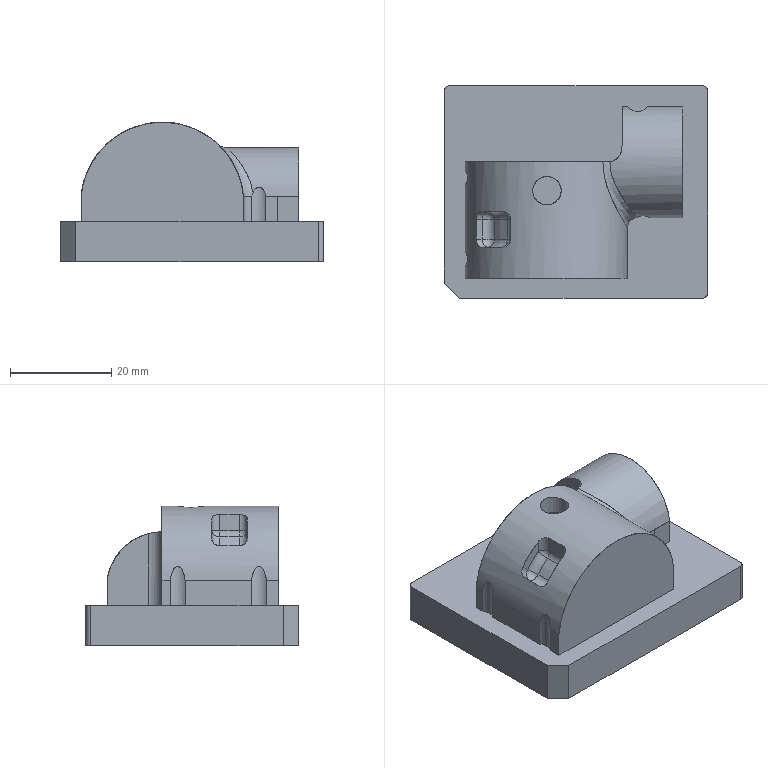NC program | PowerMill | posted with a generic post | part box 52 x 42 x 27.622 mm
Lines 8086 to 9073 of 214543:
N8183 M6
N8184 S18000 M03
N8185 G00 G90 X0.0 Y0.0
N8186 G43 Z9.8022 H2
N8187
N8188 G05 P10000 R4
N8189 X-11.2727 Y-8.4983
N8190 Z0.664
N8191 G01 Z-0.536 F3600.0
N8192 X-11.253 Y-8.5082 F6000.0
N8193 G03 X-10.9873 Y-8.4197 I0.0886 J0.1771
N8194 G01 X-10.3152 Y-7.0768
N8195 X-10.3131 Y-0.9761
N8196 X-10.3217 Y-0.4881
N8197 X-10.2511 Y0.0403
N8198 X-10.2223 Y0.1152
N8199 X-10.2021 Y0.1929
N8200 X-10.2026 Y0.2432
N8201 X-10.2153 Y0.2919
N8202 X-10.2491 Y0.39
N8203 X-10.3272 Y0.9761
N8204 X-10.2726 Y2.4403
N8205 X-10.3162 Y2.9283
N8206 X-10.3149 Y5.8566
N8207 X-10.271 Y6.3447
N8208 X-10.0887 Y6.8327
N8209 X-9.7611 Y7.2673
N8210 X-9.273 Y7.6166
N8211 X-8.7849 Y7.7804
N8212 X-8.5449 Y7.8088
N8213 X-3.2182
N8214 X-2.9283 Y7.7687
N8215 X-2.4403 Y7.5912
N8216 X-2.0533 Y7.3208
N8217 X-1.9522 Y7.217
N8218 X-1.672 Y6.8327
N8219 X-1.4899 Y6.3447
N8220 X-1.4465 Y5.8566
N8221 X-1.4524 Y3.4164
N8222 X-1.4311 Y2.9283
N8223 X-1.4486 Y2.4403
N8224 X-1.4344 Y1.4642
N8225 X-1.5424 Y0.9761
N8226 X-1.7966 Y0.4881
N8227 X-1.9197 Y0.3411
N8228 G03 X-1.915 Y0.0789 I0.1533 J-0.1284
N8229 G01 X-1.844 Y0.0
N8230 X-1.5621 Y-0.4881
N8231 X-1.4394 Y-0.9761
N8232 X-1.4309 Y-5.3686
N8233 X-1.4721 Y-11.7133
N8234 X-1.4462 Y-13.1774
N8235 X-1.4642 Y-13.5042
N8236 X-1.4978 Y-13.6655
N8237 X-1.5076 Y-16.5938
N8238 X-1.4799 Y-17.0818
N8239 X-1.5236 Y-17.5699
N8240 X-1.7078 Y-18.0579
N8241 X-1.9522 Y-18.3978
N8242 X-2.0901 Y-18.546
N8243 X-2.4403 Y-18.7916
N8244 X-2.9283 Y-18.982
N8245 X-3.4164 Y-19.0312
N8246 X-8.2969
N8247 X-8.7849 Y-18.9916
N8248 X-9.273 Y-18.8145
N8249 X-9.6626 Y-18.546
N8250 X-10.0487 Y-18.0579
N8251 X-10.2321 Y-17.5699
N8252 X-10.2757 Y-17.0818
N8253 X-10.2491 Y-16.7603
N8254 Y-13.7412
N8255 X-10.3174 Y-13.1774
N8256 X-10.3152 Y-7.0768
N8257 X-12.3194 Y-8.5465 Z-0.7339
N8258 X-12.2998 Y-8.5564
N8259 G03 X-12.0338 Y-8.4688 I0.0892 J0.1768
N8260 G01 X-11.3303 Y-7.0734
N8261 X-11.3083 Y-0.4881
N8262 X-11.341 Y0.4881
N8263 X-11.3376 Y1.9522
N8264 X-11.305 Y5.3686
N8265 X-11.3264 Y5.8566
N8266 X-11.2852 Y6.3447
N8267 X-11.1038 Y6.8327
N8268 X-10.7372 Y7.3041
N8269 X-10.2491 Y7.6361
N8270 X-9.7611 Y7.7863
N8271 X-9.5559 Y7.8088
N8272 X-2.2151
N8273 X-1.9522 Y7.776
N8274 X-1.4642 Y7.607
N8275 X-1.0506 Y7.3208
N8276 X-0.669 Y6.8327
N8277 X-0.4869 Y6.3447
N8278 X-0.4442 Y5.8566
N8279 X-0.4593 Y5.3686
N8280 X-0.4372 Y2.9283
N8281 X-0.4241 Y0.4881
N8282 X-0.4683 Y-0.4881
N8283 X-0.4694 Y-12.6894
N8284 X-0.4687 Y-12.6975
N8285 Y-12.6977
N8286 X-0.4287 Y-13.1774
N8287 X-0.4433 Y-17.0818
N8288 X-0.4874 Y-17.5699
N8289 X-0.6713 Y-18.0579
N8290 X-1.0566 Y-18.546
N8291 X-1.4642 Y-18.827
N8292 X-1.9522 Y-18.9954
N8293 X-2.4403 Y-19.0312
N8294 X-9.273
N8295 X-9.7611 Y-19.0038
N8296 X-10.2491 Y-18.8451
N8297 X-10.6981 Y-18.546
N8298 X-11.0831 Y-18.0579
N8299 X-11.2671 Y-17.5699
N8300 X-11.3123 Y-17.0818
N8301 Y-13.6655
N8302 X-11.3366 Y-13.1774
N8303 X-11.3039 Y-12.6894
N8304 Y-9.7611
N8305 X-11.3376 Y-9.273
N8306 X-11.3303 Y-7.0734
N8307 X-13.0764 Y-8.5492 Z-0.9319
N8308 X-13.0568 Y-8.5591
N8309 G03 X-12.7909 Y-8.4712 I0.089 J0.1769
N8310 G01 X-12.0869 Y-7.0716
N8311 X-12.0711 Y-0.4881
N8312 X-12.0926 Y0.4881
N8313 X-12.0688 Y1.9522
N8314 X-12.0711 Y5.3686
N8315 X-12.1008 Y5.8566
N8316 X-12.0572 Y6.3447
N8317 X-11.8757 Y6.8327
N8318 X-11.7133 Y7.0774
N8319 X-11.4951 Y7.3208
N8320 X-11.2252 Y7.5232
N8321 X-10.7372 Y7.7406
N8322 X-10.3258 Y7.8088
N8323 X-1.4166
N8324 X-0.9761 Y7.7318
N8325 X-0.4881 Y7.5019
N8326 X-0.2517 Y7.3208
N8327 X0.0 Y7.0353
N8328 X0.1291 Y6.8327
N8329 X0.3117 Y6.3447
N8330 X0.3535 Y5.8566
N8331 X0.3233 Y5.3686
N8332 X0.3174 Y2.4403
N8333 X0.3512 Y0.4881
N8334 X0.3285 Y-0.4881
N8335 Y-12.6894
N8336 X0.3501 Y-13.1774
N8337 X0.3226 Y-13.6655
N8338 Y-13.6714
N8339 X0.3364 Y-17.0818
N8340 X0.2924 Y-17.5699
N8341 X0.1097 Y-18.0579
N8342 X0.0 Y-18.2297
N8343 X-0.2743 Y-18.546
N8344 X-0.4881 Y-18.7104
N8345 X-0.9761 Y-18.9454
N8346 X-1.4642 Y-19.0295
N8347 X-2.4202 Y-19.0296
N8348 X-2.4403 Y-19.0311
N8349 X-9.273
N8350 X-9.2812 Y-19.0306
N8351 X-10.2491 Y-19.0308
N8352 X-10.7372 Y-18.9583
N8353 X-11.2252 Y-18.7393
N8354 X-11.4808 Y-18.546
N8355 X-11.7133 Y-18.2916
N8356 X-11.865 Y-18.0579
N8357 X-12.0489 Y-17.5699
N8358 X-12.0927 Y-17.0818
N8359 X-12.0773 Y-16.5938
N8360 X-12.0945 Y-13.1774
N8361 X-12.0711 Y-12.6894
N8362 Y-9.7611
N8363 X-12.0922 Y-9.273
N8364 X-12.0869 Y-7.0716
N8365 X-13.7539 Y-8.5524 Z-1.1299
N8366 X-13.7342 Y-8.5622
N8367 G03 X-13.4686 Y-8.4737 I0.0885 J0.1771
N8368 G01 X-12.7676 Y-7.0716
N8369 X-12.768 Y5.8566
N8370 X-12.7253 Y6.3447
N8371 X-12.543 Y6.8327
N8372 X-12.2013 Y7.2806
N8373 X-11.7133 Y7.6229
N8374 X-11.2252 Y7.7828
N8375 X-10.9964 Y7.8088
N8376 X-0.7671
N8377 X-0.4881 Y7.7728
N8378 X0.0 Y7.5993
N8379 X0.3964 Y7.3208
N8380 X0.7814 Y6.8327
N8381 X0.9612 Y6.3447
N8382 X1.0032 Y5.8566
N8383 X1.0097 Y0.4881
N8384 X0.9823 Y-0.4881
N8385 Y-12.6894
N8386 X0.9825 Y-12.6936
N8387 X1.0032 Y-13.1774
N8388 X0.9807 Y-13.6655
N8389 Y-16.5938
N8390 X1.0019 Y-17.0818
N8391 X0.9585 Y-17.5699
N8392 X0.7753 Y-18.0579
N8393 X0.3911 Y-18.546
N8394 X0.0 Y-18.8157
N8395 X-0.4881 Y-18.9922
N8396 X-0.9761 Y-19.0312
N8397 X-10.7372
N8398 X-11.2252 Y-19.0004
N8399 X-11.7133 Y-18.8375
N8400 X-12.1463 Y-18.546
N8401 X-12.5291 Y-18.0579
N8402 X-12.6894 Y-17.6582
N8403 X-12.7593 Y-17.0818
N8404 X-12.7343 Y-16.5938
N8405 Y-13.6655
N8406 X-12.7347 Y-13.6588
N8407 X-12.7674 Y-13.1774
N8408 X-12.7676 Y-7.0716
N8409 X-14.3135 Y-8.565 Z-1.3279
N8410 X-14.2939 Y-8.5749
N8411 G03 X-14.0278 Y-8.4877 I0.0895 J0.1766
N8412 G01 X-13.3091 Y-7.0688
N8413 X-13.3004 Y-5.3686
N8414 X-13.3058 Y5.3686
N8415 X-13.3302 Y5.8566
N8416 X-13.2882 Y6.3447
N8417 X-13.1774 Y6.6932
N8418 X-13.1083 Y6.8327
N8419 X-12.7282 Y7.3208
N8420 X-12.2013 Y7.6604
N8421 X-11.7133 Y7.7948
N8422 X-11.5628 Y7.8088
N8423 X-0.1929
N8424 X0.0 Y7.7882
N8425 X0.4881 Y7.6408
N8426 X0.9761 Y7.3146
N8427 X1.3529 Y6.8327
N8428 X1.4642 Y6.5808
N8429 X1.5353 Y6.3447
N8430 X1.5774 Y5.8566
N8431 X1.5492 Y5.3686
N8432 X1.5454 Y2.4403
N8433 X1.5729 Y0.4881
N8434 X1.5529 Y-0.4881
N8435 Y-0.4901
N8436 X1.5522 Y-6.8338
N8437 X1.5681 Y-13.1774
N8438 X1.5451 Y-13.6655
N8439 Y-13.6705
N8440 X1.5541 Y-17.0818
N8441 X1.5105 Y-17.5699
N8442 X1.3267 Y-18.0579
N8443 X0.9424 Y-18.546
N8444 X0.4881 Y-18.8479
N8445 X0.0 Y-19.0044
N8446 X-0.4881 Y-19.0312
N8447 X-11.2252
N8448 X-11.7133 Y-19.0105
N8449 X-12.2013 Y-18.8681
N8450 X-12.698 Y-18.546
N8451 X-13.0829 Y-18.0579
N8452 X-13.1774 Y-17.8526
N8453 X-13.2668 Y-17.5699
N8454 X-13.3097 Y-17.0818
N8455 X-13.2998 Y-16.5938
N8456 X-13.3155 Y-13.1774
N8457 X-13.2967 Y-12.6894
N8458 Y-9.7611
N8459 X-13.3205 Y-9.273
N8460 X-13.3091 Y-7.0688
N8461 X-14.8404 Y-8.5748 Z-1.5258
N8462 X-14.8208 Y-8.5847
N8463 G03 X-14.5551 Y-8.4963 I0.0887 J0.1771
N8464 G01 X-13.8402 Y-7.0685
N8465 X-13.8331 Y5.8566
N8466 X-13.7893 Y6.3447
N8467 X-13.6075 Y6.8327
N8468 X-13.2258 Y7.3208
N8469 X-12.6894 Y7.6636
N8470 X-12.2013 Y7.7962
N8471 X-11.6919 Y7.7967
N8472 X-11.5628 Y7.8088
N8473 X-0.1929
N8474 X-0.1863 Y7.8085
N8475 X-0.1796 Y7.8084
N8476 X0.3068 Y7.8088
N8477 X0.4881 Y7.7899
N8478 X0.9761 Y7.6461
N8479 X1.4711 Y7.3208
N8480 X1.8528 Y6.8327
N8481 X1.9522 Y6.61
N8482 X2.0345 Y6.3447
N8483 X2.0765 Y5.8566
N8484 X2.085 Y0.4881
N8485 X2.0547 Y-0.4881
N8486 Y-12.6894
N8487 X2.085 Y-13.1774
N8488 X2.0855 Y-17.0818
N8489 X2.0407 Y-17.5699
N8490 X1.9522 Y-17.8552
N8491 X1.8579 Y-18.0579
N8492 X1.4736 Y-18.546
N8493 X0.9761 Y-18.869
N8494 X0.4881 Y-19.0104
N8495 X0.0 Y-19.0312
N8496 X-11.7133
N8497 X-12.2013 Y-19.0166
N8498 X-12.6894 Y-18.8886
N8499 X-13.1774 Y-18.5908
N8500 X-13.6127 Y-18.0579
N8501 X-13.7977 Y-17.5699
N8502 X-13.842 Y-17.0818
N8503 X-13.8432 Y-13.1774
N8504 X-13.8222 Y-12.6894
N8505 Y-9.7611
N8506 X-13.8414 Y-9.273
N8507 X-13.8402 Y-7.0685
N8508 X-15.2983 Y-8.5761 Z-1.7238
N8509 X-15.2787 Y-8.586
N8510 G03 X-15.013 Y-8.4975 I0.0886 J0.1771
N8511 G01 X-14.2981 Y-7.0684
N8512 X-14.2968 Y-1.4642
N8513 X-14.2849 Y0.9761
N8514 X-14.3027 Y5.8566
N8515 X-14.2625 Y6.3447
N8516 X-14.0801 Y6.8327
N8517 X-13.6982 Y7.3208
N8518 X-13.1774 Y7.658
N8519 X-12.6894 Y7.7939
N8520 X-12.5336 Y7.8088
N8521 X0.7777
N8522 X0.9761 Y7.7873
N8523 X1.4642 Y7.6377
N8524 X1.9426 Y7.3208
N8525 X2.3239 Y6.8327
N8526 X2.4403 Y6.5697
N8527 X2.506 Y6.3447
N8528 X2.5483 Y5.8566
N8529 X2.538 Y2.9275
N8530 Y2.9267
N8531 X2.5511 Y0.0
N8532 X2.5517 Y-13.1774
N8533 X2.5198 Y-13.6655
N8534 X2.5305 Y-17.0818
N8535 X2.487 Y-17.5699
N8536 X2.3032 Y-18.0579
N8537 X1.9189 Y-18.546
N8538 X1.4642 Y-18.8489
N8539 X0.9761 Y-19.0045
N8540 X0.4881 Y-19.0312
N8541 X-12.2013
N8542 X-12.6894 Y-19.0106
N8543 X-13.1774 Y-18.8693
N8544 X-13.6744 Y-18.546
N8545 X-14.0587 Y-18.0579
N8546 X-14.1535 Y-17.8499
N8547 X-14.2424 Y-17.5699
N8548 X-14.2861 Y-17.0818
N8549 X-14.2737 Y-13.6655
N8550 X-14.2941 Y-13.1774
N8551 X-14.2985 Y-9.273
N8552 X-14.2981 Y-7.0684
N8553 X-15.7274 Y-8.5633 Z-1.9218
N8554 X-15.7078 Y-8.5732
N8555 G03 X-15.4418 Y-8.4857 I0.0892 J0.1767
N8556 G01 X-14.7257 Y-7.0668
N8557 X-14.7083 Y-2.4403
N8558 X-14.7155 Y5.8566
N8559 X-14.6729 Y6.3447
N8560 X-14.4913 Y6.8327
N8561 X-14.1535 Y7.2779
N8562 X-13.6655 Y7.622
N8563 X-13.1774 Y7.782
N8564 X-12.6894 Y7.8113
N8565 X1.2014 Y7.8088
N8566 X1.4642 Y7.7759
N8567 X1.9522 Y7.6057
N8568 X2.4403 Y7.2488
N8569 X2.7466 Y6.8327
N8570 X2.9288 Y6.3447
N8571 X2.9705 Y5.8566
N8572 X2.9532 Y5.3686
N8573 Y5.365
N8574 X2.9593 Y0.9761
N8575 X2.953 Y-0.4881
N8576 Y-12.6894
N8577 X2.9532 Y-12.6932
N8578 X2.9715 Y-13.1774
N8579 X2.9684 Y-17.0818
N8580 X2.9249 Y-17.5699
N8581 X2.741 Y-18.0579
N8582 X2.3567 Y-18.546
N8583 X1.9522 Y-18.8241
N8584 X1.4642 Y-18.995
N8585 X0.9761 Y-19.0312
N8586 X-12.6894
N8587 X-13.1774 Y-19.003
N8588 X-13.6655 Y-18.8465
N8589 X-14.1123 Y-18.546
N8590 X-14.4966 Y-18.0579
N8591 X-14.6802 Y-17.5699
N8592 X-14.7239 Y-17.0818
N8593 X-14.7073 Y-10.2491
N8594 X-14.734 Y-9.273
N8595 X-14.7257 Y-7.0668
N8596 X-15.8149 Y-8.6426 Z-2.1198
N8597 X-15.7952 Y-8.6524
N8598 G03 X-15.5295 Y-8.564 I0.0886 J0.177
N8599 G01 X-14.78 Y-7.0668
N8600 X-14.7793 Y-5.66
N8601 X-14.7869 Y-5.6054
N8602 X-14.809 Y-5.5549
N8603 X-14.9239 Y-5.3686
N8604 X-15.0957 Y-4.8805
N8605 X-15.1296 Y-4.6055
N8606 X-15.1254 Y-3.9044
N8607 Y-3.9038
N8608 X-15.1253 Y5.8566
N8609 X-15.0855 Y6.3447
N8610 X-14.9031 Y6.8327
N8611 X-14.6416 Y7.1993
N8612 X-14.5225 Y7.3208
N8613 X-14.1535 Y7.583
N8614 X-13.6655 Y7.7668
N8615 X-13.1774 Y7.8113
N8616 X-12.6899 Y7.8112
N8617 X-12.6894 Y7.8113
N8618 X-9.7699 Y7.8107
N8619 X1.6056 Y7.8088
N8620 X1.9522 Y7.7574
N8621 X2.4403 Y7.5615
N8622 X2.7696 Y7.3208
N8623 X2.9283 Y7.1559
N8624 X3.1516 Y6.8327
N8625 X3.3342 Y6.3447
N8626 X3.3743 Y5.8566
N8627 X3.377 Y2.9283
N8628 X3.3555 Y-0.4881
N8629 Y-12.6894
N8630 X3.3741 Y-13.1774
N8631 X3.3657 Y-17.0818
N8632 X3.3206 Y-17.5699
N8633 X3.1362 Y-18.0579
N8634 X2.9283 Y-18.3607
N8635 X2.7522 Y-18.546
N8636 X2.4403 Y-18.7733
N8637 X1.9522 Y-18.9728
N8638 X1.4642 Y-19.0312
N8639 X-13.1774
N8640 X-13.6655 Y-18.9841
N8641 X-14.1535 Y-18.7977
N8642 X-14.5075 Y-18.546
N8643 X-14.6416 Y-18.4102
N8644 X-14.8918 Y-18.0579
N8645 X-15.0756 Y-17.5699
N8646 X-15.1206 Y-17.0818
N8647 X-15.1314 Y-10.2491
N8648 X-15.0501 Y-9.7611
N8649 X-14.8016 Y-9.2556
N8650 X-14.7862 Y-9.2127
N8651 X-14.781 Y-9.1675
N8652 X-14.78 Y-7.0668
N8653 X-16.0588 Y-9.1299 Z-2.3177
N8654 X-16.0391 Y-9.1398
N8655 G03 X-15.7735 Y-9.0513 I0.0886 J0.1771
N8656 G01 X-14.7799 Y-7.0668
N8657 X-14.7793 Y-5.7347
N8658 X-14.7957 Y-5.6571
N8659 X-14.8409 Y-5.592
N8660 X-15.074 Y-5.3686
N8661 X-15.3674 Y-4.8805
N8662 X-15.4919 Y-4.3925
N8663 X-15.4877 Y0.7321
N8664 X-15.4943 Y5.8566
N8665 X-15.4522 Y6.3447
N8666 X-15.2701 Y6.8327
N8667 X-15.1296 Y7.0508
N8668 X-14.8888 Y7.3208
N8669 X-14.6416 Y7.511
N8670 X-14.1535 Y7.7341
N8671 X-13.724 Y7.8088
N8672 X-13.2038
N8673 X-13.1774 Y7.8113
N8674 X-12.6899 Y7.8112
N8675 X-12.6894
N8676 X-9.7699 Y7.8107
N8677 X1.305 Y7.8088
N8678 X1.974
N8679 X2.4403 Y7.7235
N8680 X2.9283 Y7.4859
N8681 X3.139 Y7.3208
N8682 X3.4164 Y6.9992
N8683 X3.5203 Y6.8327
N8684 X3.7021 Y6.3447
N8685 X3.7453 Y5.8566
N8686 X3.7327 Y5.3686
N8687 X3.7465 Y0.0
N8688 X3.7477 Y-13.1774
N8689 X3.7222 Y-13.6655
N8690 X3.7297 Y-17.0818
N8691 X3.687 Y-17.5699
N8692 X3.5033 Y-18.0579
N8693 X3.4164 Y-18.1987
N8694 X3.1189 Y-18.546
N8695 X2.9283 Y-18.697
N8696 X2.4403 Y-18.9391
N8697 X1.9522 Y-19.0288
N8698 X1.4832
N8699 X1.4642 Y-19.0311
N8700 X-13.1774
N8701 X-13.1883 Y-19.0301
N8702 X-13.6655
N8703 X-14.1535 Y-18.9518
N8704 X-14.6416 Y-18.7244
N8705 X-14.8747 Y-18.546
N8706 X-15.1296 Y-18.2582
N8707 X-15.259 Y-18.0579
N8708 X-15.4426 Y-17.5699
N8709 X-15.4862 Y-17.0818
N8710 X-15.4777 Y-16.5938
N8711 X-15.5061 Y-10.7372
N8712 X-15.4597 Y-10.2491
N8713 X-15.2769 Y-9.7611
N8714 X-15.1296 Y-9.5298
N8715 X-14.837 Y-9.2325
N8716 X-14.8099 Y-9.198
N8717 X-14.8003 Y-9.1782
N8718 X-14.7859 Y-9.1367
N8719 X-14.7809 Y-9.0931
N8720 X-14.7799 Y-7.0668
N8721 X-16.8357 Y-10.6818 Z-2.5157
N8722 X-16.816 Y-10.6917
N8723 G03 X-16.5503 Y-10.6032 I0.0886 J0.1771
N8724 G01 X-14.7799 Y-7.0668
N8725 X-14.7793 Y-5.8144
N8726 X-14.7812 Y-5.8007
N8727 X-14.8135 Y-5.703
N8728 X-14.8912 Y-5.6355
N8729 X-15.2602 Y-5.3686
N8730 X-15.6177 Y-4.9112
N8731 X-15.8131 Y-4.3925
N8732 X-15.8552 Y-3.9044
N8733 X-15.8311 Y-1.9522
N8734 X-15.836 Y5.8566
N8735 X-15.7939 Y6.3447
N8736 X-15.6118 Y6.8327
N8737 X-15.2305 Y7.3208
N8738 X-15.1296 Y7.4058
N8739 X-14.6416 Y7.6849
N8740 X-14.1535 Y7.8007
N8741 X-13.7695 Y7.8009
N8742 X-13.724 Y7.8088
N8743 X-13.2038
N8744 X-13.1774 Y7.8112
N8745 X-12.6899 Y7.8111
N8746 X-12.6894 Y7.8112
N8747 X-9.7699 Y7.8106
N8748 X1.305 Y7.8088
N8749 X1.974
N8750 X1.9747 Y7.8087
N8751 X2.3243 Y7.8088
N8752 X2.9283 Y7.6743
N8753 X3.4898 Y7.3208
N8754 X3.8697 Y6.8327
N8755 X4.0525 Y6.3447
N8756 X4.0943 Y5.8566
N8757 X4.0768 Y5.3686
N8758 X4.0818 Y0.9761
N8759 X4.0774 Y-0.4881
N8760 Y-12.6894
N8761 X4.0964 Y-17.0818
N8762 X4.055 Y-17.5699
N8763 X3.9044 Y-17.9918
N8764 X3.4869 Y-18.546
N8765 X2.9283 Y-18.8956
N8766 X2.4403 Y-19.0187
N8767 X1.9522 Y-19.0312
N8768 X-13.6655
N8769 X-14.1535 Y-19.0232
N8770 X-14.6416 Y-18.9119
N8771 X-15.1296 Y-18.64
N8772 X-15.2424 Y-18.546
N8773 X-15.6177 Y-18.0734
N8774 X-15.8104 Y-17.5699
N8775 X-15.8538 Y-17.0818
N8776 X-15.8346 Y-16.5938
N8777 X-15.8303 Y-12.6894
N8778 X-15.8529 Y-10.7372
N8779 X-15.7624 Y-10.2491
N8780 X-15.6177 Y-9.9165
N8781 X-15.5226 Y-9.7611
N8782 X-15.1296 Y-9.3475
N8783 X-14.8743 Y-9.1899
N8784 X-14.811 Y-9.1278
N8785 X-14.7809 Y-9.0444
N8786 X-14.7799 Y-7.0668
N8787 X-16.1848 Y-8.57 Z-2.7137
N8788 X-16.1652 Y-8.5799
N8789 G03 X-15.8995 Y-8.4915 I0.0887 J0.1771
N8790 G01 X-14.7794 Y-6.2542
N8791 X-14.7793 Y-5.9105
N8792 X-14.793 Y-5.8038
N8793 X-14.857 Y-5.7174
N8794 X-14.9101 Y-5.688
N8795 X-14.9242 Y-5.6828
N8796 X-15.1296 Y-5.607
N8797 X-15.5051 Y-5.3686
N8798 X-15.6177 Y-5.2674
N8799 X-15.9258 Y-4.8805
N8800 X-16.1057 Y-4.4641
N8801 X-16.1866 Y-3.9044
N8802 X-16.1777 Y5.8566
N8803 X-16.1356 Y6.3447
N8804 X-15.9535 Y6.8327
N8805 X-15.6177 Y7.2759
N8806 X-15.1296 Y7.6217
N8807 X-14.6416 Y7.7816
N8808 X-14.1535 Y7.8113
N8809 X-12.6896 Y7.8111
N8810 X-12.6894
N8811 X-12.2274 Y7.811
N8812 X2.6576 Y7.8088
N8813 X2.9283 Y7.7745
N8814 X3.4164 Y7.6034
N8815 X3.8234 Y7.3208
N8816 X4.2039 Y6.8327
N8817 X4.3862 Y6.3447
N8818 X4.4288 Y5.8566
N8819 X4.4317 Y0.4881
N8820 X4.4083 Y-0.4881
N8821 Y-12.6894
N8822 X4.43 Y-13.1774
N8823 X4.4299 Y-17.0818
N8824 X4.3925 Y-17.5296
N8825 X4.2008 Y-18.0579
N8826 X3.8165 Y-18.546
N8827 X3.4164 Y-18.8229
N8828 X2.9283 Y-18.9943
N8829 X2.4403 Y-19.0312
N8830 X-14.1535
N8831 X-14.6416 Y-19.0018
N8832 X-15.1296 Y-18.8437
N8833 X-15.5721 Y-18.546
N8834 X-15.955 Y-18.0579
N8835 X-16.1394 Y-17.5699
N8836 X-16.1852 Y-17.0818
N8837 X-16.1876 Y-13.9095
N8838 X-16.1785 Y-10.7372
N8839 X-16.068 Y-10.2491
N8840 X-15.7988 Y-9.7611
N8841 X-15.6177 Y-9.5586
N8842 X-15.2386 Y-9.273
N8843 X-14.9043 Y-9.1379
N8844 X-14.8206 Y-9.0742
N8845 X-14.7808 Y-8.9768
N8846 X-14.7794 Y-6.2542
N8847 X-16.5683 Y-6.1914 Z-2.9117
N8848 X-16.5464 Y-6.1928
N8849 G03 X-16.3368 Y-6.0071 I0.012 J0.1977
N8850 G01 X-16.2629 Y-4.79
N8851 X-16.4324 Y-4.3925
N8852 X-16.4953 Y-3.9044
N8853 X-16.4968 Y5.8566
N8854 X-16.4532 Y6.3447
N8855 X-16.2708 Y6.8327
N8856 X-16.1057 Y7.085
N8857 X-15.8894 Y7.3208
N8858 X-15.6177 Y7.5262
N8859 X-15.1296 Y7.7419
N8860 X-14.7236 Y7.8088
N8861 X-14.1931
N8862 X-14.1535 Y7.8113
N8863 X-12.6896 Y7.811
N8864 X-12.6894 Y7.8111
N8865 X-12.2274 Y7.811
N8866 X2.3159 Y7.8088
N8867 X2.9695
N8868 X3.4164 Y7.7302
N8869 X3.9044 Y7.5003
N8870 X4.1343 Y7.3208
N8871 X4.3925 Y7.0271
N8872 X4.5157 Y6.8327
N8873 X4.6978 Y6.3447
N8874 X4.7405 Y5.8566
N8875 X4.7393 Y-12.2013
N8876 X4.7248 Y-13.6655
N8877 X4.7283 Y-17.0818
N8878 X4.6846 Y-17.5699
N8879 X4.501 Y-18.0579
N8880 X4.3925 Y-18.2323
N8881 X4.1164 Y-18.546
N8882 X3.9044 Y-18.7114
N8883 X3.4164 Y-18.9452
N8884 X2.9283 Y-19.0296
N8885 X2.4595 Y-19.0297
N8886 X2.4403 Y-19.0311
N8887 X-14.1535
N8888 X-14.1573 Y-19.031
N8889 X-14.161
N8890 X-14.6416
N8891 X-15.1296 Y-18.9573
N8892 X-15.6177 Y-18.7385
N8893 X-15.8722 Y-18.546
N8894 X-16.1057 Y-18.2896
N8895 X-16.257 Y-18.0579
N8896 X-16.4401 Y-17.5699
N8897 X-16.4839 Y-17.0818
N8898 X-16.4861 Y-10.7372
N8899 X-16.3691 Y-10.2491
N8900 X-16.0907 Y-9.7611
N8901 X-15.6177 Y-9.3407
N8902 X-15.503 Y-9.273
N8903 X-15.1296 Y-9.1241
N8904 X-14.9441 Y-9.0905
N8905 G03 X-14.7807 Y-8.9123 I-0.0357 J0.1968
N8906 G01 X-14.7793 Y-6.1448
N8907 Y-5.9414
N8908 G03 X-14.9432 Y-5.7446 I-0.2 J0.0001
N8909 G01 X-15.1296 Y-5.7105
N8910 X-15.6177 Y-5.4954
N8911 X-15.7964 Y-5.3686
N8912 X-16.1057 Y-5.0505
N8913 X-16.2243 Y-4.8805
N8914 X-16.2629 Y-4.79
N8915 X-16.8452 Y-6.2207 Z-3.1096
N8916 X-16.8232 Y-6.222
N8917 G03 X-16.6136 Y-6.0364 I0.012 J0.1976
N8918 G01 X-16.54 Y-4.8258
N8919 X-16.7247 Y-4.3925
N8920 X-16.7877 Y-3.9044
N8921 X-16.7815 Y5.8566
N8922 X-16.7395 Y6.3447
N8923 X-16.5938 Y6.759
N8924 X-16.1763 Y7.3208
N8925 X-15.6177 Y7.6722
N8926 X-15.1296 Y7.7988
N8927 X-15.0112 Y7.8088
N8928 X-14.7315 Y7.8086
N8929 X-14.7275 Y7.8087
N8930 X-14.7236 Y7.8088
N8931 X-14.1931
N8932 X-14.1535 Y7.8112
N8933 X-12.6896 Y7.811
N8934 X-12.6894
N8935 X-12.2274 Y7.8109
N8936 X2.3159 Y7.8088
N8937 X2.9695
N8938 X3.0442 Y7.7957
N8939 X3.4164 Y7.7954
N8940 X3.9044 Y7.6613
N8941 X4.3925 Y7.3589
N8942 X4.817 Y6.8327
N8943 X4.9991 Y6.3447
N8944 X5.0413 Y5.8566
N8945 X5.0236 Y5.3686
N8946 X5.0305 Y0.0
N8947 Y-12.6894
N8948 X5.0197 Y-16.5938
N8949 X5.0419 Y-17.0818
N8950 X4.9976 Y-17.5699
N8951 X4.8145 Y-18.0579
N8952 X4.4287 Y-18.546
N8953 X3.9044 Y-18.8821
N8954 X3.4164 Y-19.0142
N8955 X2.9283 Y-19.0312
N8956 X-14.6416
N8957 X-15.1296 Y-19.0201
N8958 X-15.6177 Y-18.8996
N8959 X-16.1057 Y-18.6135
N8960 X-16.1858 Y-18.546
N8961 X-16.5701 Y-18.0579
N8962 X-16.7529 Y-17.5699
N8963 X-16.7974 Y-17.0818
N8964 X-16.7753 Y-16.5938
N8965 X-16.7784 Y-10.7372
N8966 X-16.6615 Y-10.2491
N8967 X-16.5938 Y-10.096
N8968 X-16.3826 Y-9.7611
N8969 X-16.1057 Y-9.4812
N8970 X-15.7954 Y-9.273
N8971 X-15.6177 Y-9.1915
N8972 X-15.1296 Y-9.0675
N8973 X-14.9718 Y-9.0616
N8974 G03 X-14.7806 Y-8.8841 I-0.0076 J0.1999
N8975 G01 X-14.7793 Y-6.1161
N8976 Y-5.9739
N8977 G03 X-14.9722 Y-5.7741 I-0.2 J0.0
N8978 G01 X-15.1296 Y-5.7684
N8979 X-15.6177 Y-5.6438
N8980 X-16.0889 Y-5.3686
N8981 X-16.5167 Y-4.8805
N8982 X-16.54 Y-4.8258
N8983 X-17.1306 Y-6.2387 Z-3.3076
N8984 X-17.1086 Y-6.24
N8985 G03 X-16.899 Y-6.0544 I0.012 J0.1976
N8986 G01 X-16.8252 Y-4.8426
N8987 X-17.0171 Y-4.3925
N8988 X-17.0801 Y-3.9044
N8989 X-17.074 Y5.8566
N8990 X-17.032 Y6.3447
N8991 X-16.8499 Y6.8327
N8992 X-16.5938 Y7.1933
N8993 X-16.4684 Y7.3208
N8994 X-16.1057 Y7.5792
N8995 X-15.6177 Y7.7644
N8996 X-15.1296 Y7.8113
N8997 X3.5535 Y7.8088
N8998 X3.9044 Y7.7565
N8999 X4.3925 Y7.5593
N9000 X4.7186 Y7.3208
N9001 X4.8805 Y7.1512
N9002 X5.1014 Y6.8327
N9003 X5.2818 Y6.3447
N9004 X5.324 Y5.8566
N9005 X5.3075 Y-0.4881
N9006 Y-12.6894
N9007 X5.3157 Y-17.0818
N9008 X5.2718 Y-17.5699
N9009 X5.088 Y-18.0579
N9010 X4.8805 Y-18.3592
N9011 X4.7046 Y-18.546
N9012 X4.3925 Y-18.7739
N9013 X3.9044 Y-18.9732
N9014 X3.4164 Y-19.0312
N9015 X-15.1296
N9016 X-15.6177 Y-18.9842
N9017 X-16.1057 Y-18.7976
N9018 X-16.4592 Y-18.546
N9019 X-16.5938 Y-18.408
N9020 X-16.8435 Y-18.0579
N9021 X-17.0282 Y-17.5699
N9022 X-17.0716 Y-17.0818
N9023 X-17.0708 Y-10.7372
N9024 X-16.954 Y-10.2491
N9025 X-16.6745 Y-9.7611
N9026 X-16.5938 Y-9.6671
N9027 X-16.1057 Y-9.2836
N9028 X-15.6177 Y-9.0994
N9029 X-15.1296 Y-9.0544
N9030 X-14.9801 Y-9.0543
N9031 G03 X-14.7806 Y-8.8462 I0.0002 J0.1995
N9032 G01 X-14.7796 Y-6.7704
N9033 X-14.7793 Y-5.9809
N9034 G03 X-14.9791 Y-5.7809 I-0.2 J0.0
N9035 G01 X-15.1296 Y-5.7807
N9036 X-15.6177 Y-5.7351
N9037 X-16.1057 Y-5.5517
N9038 X-16.3814 Y-5.3686
N9039 X-16.5938 Y-5.1679
N9040 X-16.8091 Y-4.8805
N9041 X-16.8252 Y-4.8426
N9042 X-17.3981 Y-6.2498 Z-3.5056
N9043 X-17.3761 Y-6.2511
N9044 G03 X-17.167 Y-6.0648 I0.0114 J0.1977
N9045 G01 X-17.097 Y-4.854
N9046 X-17.2953 Y-4.3925
N9047 X-17.3585 Y-3.9044
N9048 X-17.3483 Y0.9761
N9049 X-17.3501 Y5.8566
N9050 X-17.3076 Y6.3447
N9051 X-17.1262 Y6.8327
N9052 X-16.7449 Y7.3208
N9053 X-16.5938 Y7.4441
N9054 X-16.1057 Y7.7036
N9055 X-15.6177 Y7.8057
N9056 X-15.1867 Y7.8058
N9057 X-15.1296 Y7.8113
N9058 X3.5331 Y7.8088
N9059 X3.8279
N9060 X4.3925 Y7.6904
N9061 X4.8805 Y7.4162
N9062 X4.9944 Y7.3208
N9063 X5.3686 Y6.8425
N9064 X5.558 Y6.3447
N9065 X5.6017 Y5.8566
N9066 X5.5846 Y0.0
N9067 Y-12.6894
N9068 X5.5974 Y-17.0818
N9069 X5.5522 Y-17.5699
N9070 X5.3686 Y-18.0575
N9071 X4.9843 Y-18.546
N9072 X4.8805 Y-18.6321
N9073 X4.3925 Y-18.9076
N9074 X3.9044 Y-19.0226
N9075 X3.4164 Y-19.0312
N9076 X-15.1296
N9077 X-15.6177 Y-19.0259
N9078 X-16.1057 Y-18.9238
N9079 X-16.5938 Y-18.6649
N9080 X-16.7396 Y-18.546
N9081 X-17.0818 Y-18.1292
N9082 X-17.3075 Y-17.5699
N9083 X-17.3527 Y-17.0818
N9084 X-17.3483 Y-10.7372
N9085 X-17.2315 Y-10.2491
N9086 X-17.0818 Y-9.9477
N9087 X-16.9523 Y-9.7611
N9088 X-16.5938 Y-9.4173
N9089 X-16.3658 Y-9.273
N9090 X-16.1057 Y-9.1591
N9091 X-15.6177 Y-9.0588
N9092 X-15.2691 Y-9.0589
N9093 X-14.9208 Y-9.0454
N9094 G03 X-14.7805 Y-8.8675 I-0.0593 J0.1911
N9095 G01 X-14.7796 Y-7.011
N9096 X-14.7793 Y-5.9919
N9097 X-14.7803 Y-5.972
N9098 X-14.7833 Y-5.9524
N9099 G03 X-14.9791 Y-5.7808 I-0.194 J-0.0238
N9100 G01 X-15.1296 Y-5.7807
N9101 X-15.1504 Y-5.7787
N9102 X-15.6177 Y-5.7758
N9103 X-16.1057 Y-5.6759
N9104 X-16.5938 Y-5.4183
N9105 X-17.0818 Y-4.8892
N9106 X-17.097 Y-4.854
N9107 X-17.6681 Y-6.2269 Z-3.7036
N9108 X-17.6461 Y-6.2283
N9109 G03 X-17.4363 Y-6.0428 I0.0121 J0.1976
N9110 G01 X-17.362 Y-4.8317
N9111 X-17.5489 Y-4.3925
N9112 X-17.6123 Y-3.9044
N9113 X-17.6127 Y5.8566
N9114 X-17.5699 Y6.3408
N9115 X-17.3872 Y6.8327
N9116 X-17.0818 Y7.2464
N9117 X-16.5938 Y7.6052
N9118 X-16.1057 Y7.7757
N9119 X-15.6177 Y7.8113
N9120 X4.0859 Y7.8088
N9121 X4.3925 Y7.7663
N9122 X4.8805 Y7.5847
N9123 X5.2508 Y7.3208
N9124 X5.3686 Y7.2002
N9125 X5.6321 Y6.8327
N9126 X5.8137 Y6.3447
N9127 X5.8562 Y5.8566
N9128 X5.8617 Y0.0
N9129 Y-12.6894
N9130 X5.8566 Y-13.1965
N9131 X5.8548 Y-17.0818
N9132 X5.8107 Y-17.5699
N9133 X5.6274 Y-18.0579
N9134 X5.3686 Y-18.4205
N9135 X5.2431 Y-18.546
N9136 X4.8805 Y-18.8035
N9137 X4.3925 Y-18.9857
N9138 X3.9044 Y-19.0312
N9139 X-15.6177
N9140 X-16.1057 Y-18.9942
N9141 X-16.5938 Y-18.8245
N9142 X-16.999 Y-18.546
N9143 X-17.383 Y-18.0579
N9144 X-17.5664 Y-17.5699
N9145 X-17.6101 Y-17.0818
N9146 X-17.6029 Y-10.7372
N9147 X-17.5699 Y-10.5321
N9148 X-17.4862 Y-10.2491
N9149 X-17.2055 Y-9.7611
N9150 X-17.0818 Y-9.6198
N9151 X-16.6196 Y-9.273
N9152 X-16.1057 Y-9.0902
N9153 X-15.6177 Y-9.0544
N9154 X-14.9801 Y-9.0543
N9155 G03 X-14.7805 Y-8.8453 I0.0001 J0.1998
N9156 G01 X-14.7797 Y-7.2481
N9157 X-14.7793 Y-5.9811
N9158 G03 X-14.9792 Y-5.781 I-0.2 J0.0001
N9159 G01 X-15.6177 Y-5.7807
N9160 X-16.1057 Y-5.7451
N9161 X-16.5938 Y-5.5752
N9162 X-16.9127 Y-5.3686
N9163 X-17.0818 Y-5.2144
N9164 X-17.3412 Y-4.8805
N9165 X-17.362 Y-4.8317
N9166 X-17.8599 Y-6.3617 Z-3.9015
N9167 X-17.8379 Y-6.3627
N9168 G03 X-17.6308 Y-6.1743 I0.0093 J0.1978
N9169 G01 X-17.5713 Y-4.9135
N9170 X-17.8017 Y-4.3925